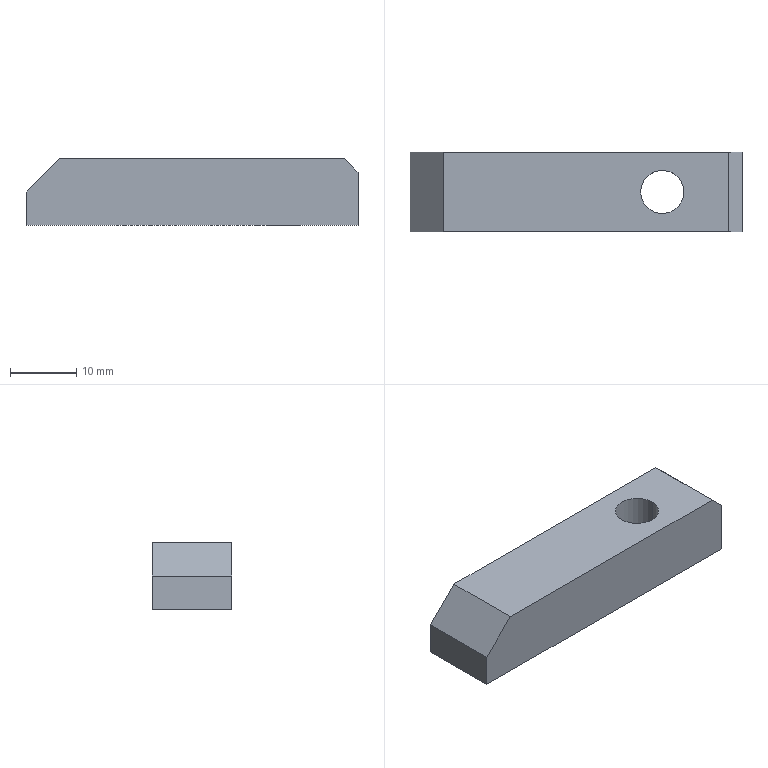Part | SolidWorks | features Chamfer 1, Extrusion 1, HoleWzd 1 | 1 solid | 10 faces | box 50 x 12 x 10 mm | volume 5494 mm3 | plane 8 | cylinder 2 | commonest cylinder face diameters 6.5 x2
STEP:
#1=CARTESIAN_POINT('',(9.75,0.,-5.));
#2=VERTEX_POINT('',#1);
#3=CARTESIAN_POINT('',(16.25,0.,-5.));
#4=VERTEX_POINT('',#3);
#5=CARTESIAN_POINT('',(13.,0.,-5.));
#6=DIRECTION('',(0.,0.,1.));
#7=DIRECTION('',(1.,0.,0.));
#8=AXIS2_PLACEMENT_3D('',#5,#6,#7);
#9=CIRCLE('',#8,3.25);
#10=EDGE_CURVE('',#2,#4,#9,.T.);
#11=ORIENTED_EDGE('',*,*,#10,.F.);
#12=CARTESIAN_POINT('',(9.75,0.,5.));
#13=VERTEX_POINT('',#12);
#14=CARTESIAN_POINT('',(9.75,0.,5.));
#15=DIRECTION('',(0.,0.,1.));
#16=VECTOR('',#15,1000.);
#17=LINE('',#14,#16);
#18=EDGE_CURVE('',#2,#13,#17,.T.);
#19=ORIENTED_EDGE('',*,*,#18,.T.);
#20=CARTESIAN_POINT('',(16.25,0.,5.));
#21=VERTEX_POINT('',#20);
#22=CARTESIAN_POINT('',(13.,0.,5.));
#23=DIRECTION('',(0.,0.,1.));
#24=DIRECTION('',(1.,0.,0.));
#25=AXIS2_PLACEMENT_3D('',#22,#23,#24);
#26=CIRCLE('',#25,3.25);
#27=EDGE_CURVE('',#13,#21,#26,.T.);
#28=ORIENTED_EDGE('',*,*,#27,.T.);
#29=CARTESIAN_POINT('',(16.25,0.,5.));
#30=DIRECTION('',(0.,0.,1.));
#31=VECTOR('',#30,1000.);
#32=LINE('',#29,#31);
#33=EDGE_CURVE('',#4,#21,#32,.T.);
#34=ORIENTED_EDGE('',*,*,#33,.F.);
#35=EDGE_LOOP('',(#11,#19,#28,#34));
#36=FACE_OUTER_BOUND('',#35,.T.);
#37=CARTESIAN_POINT('',(13.,0.,5.));
#38=DIRECTION('',(0.,0.,1.));
#39=DIRECTION('',(1.,0.,0.));
#40=AXIS2_PLACEMENT_3D('',#37,#38,#39);
#41=CYLINDRICAL_SURFACE('',#40,3.25);
#42=ADVANCED_FACE('',(#36),#41,.F.);
#43=CARTESIAN_POINT('',(-25.,6.,0.));
#44=VERTEX_POINT('',#43);
#45=CARTESIAN_POINT('',(-20.,6.,5.));
#46=VERTEX_POINT('',#45);
#47=CARTESIAN_POINT('',(-25.,6.,0.));
#48=DIRECTION('',(0.7071,0.,0.7071));
#49=VECTOR('',#48,1000.);
#50=LINE('',#47,#49);
#51=EDGE_CURVE('',#44,#46,#50,.T.);
#52=ORIENTED_EDGE('',*,*,#51,.F.);
#53=CARTESIAN_POINT('',(-25.,-6.,0.));
#54=VERTEX_POINT('',#53);
#55=CARTESIAN_POINT('',(-25.,-6.,0.));
#56=DIRECTION('',(0.,1.,0.));
#57=VECTOR('',#56,1000.);
#58=LINE('',#55,#57);
#59=EDGE_CURVE('',#54,#44,#58,.T.);
#60=ORIENTED_EDGE('',*,*,#59,.F.);
#61=CARTESIAN_POINT('',(-20.,-6.,5.));
#62=VERTEX_POINT('',#61);
#63=CARTESIAN_POINT('',(-25.,-6.,0.));
#64=DIRECTION('',(0.7071,0.,0.7071));
#65=VECTOR('',#64,1000.);
#66=LINE('',#63,#65);
#67=EDGE_CURVE('',#54,#62,#66,.T.);
#68=ORIENTED_EDGE('',*,*,#67,.T.);
#69=CARTESIAN_POINT('',(-20.,-6.,5.));
#70=DIRECTION('',(0.,1.,0.));
#71=VECTOR('',#70,1000.);
#72=LINE('',#69,#71);
#73=EDGE_CURVE('',#62,#46,#72,.T.);
#74=ORIENTED_EDGE('',*,*,#73,.T.);
#75=EDGE_LOOP('',(#52,#60,#68,#74));
#76=FACE_OUTER_BOUND('',#75,.T.);
#77=CARTESIAN_POINT('',(-25.,-6.,0.));
#78=DIRECTION('',(-0.7071,0.,0.7071));
#79=DIRECTION('',(0.7071,0.,0.7071));
#80=AXIS2_PLACEMENT_3D('',#77,#78,#79);
#81=PLANE('',#80);
#82=ADVANCED_FACE('',(#76),#81,.T.);
#83=CARTESIAN_POINT('',(-25.,6.,-5.));
#84=VERTEX_POINT('',#83);
#85=CARTESIAN_POINT('',(-25.,6.,-5.));
#86=DIRECTION('',(0.,0.,1.));
#87=VECTOR('',#86,1000.);
#88=LINE('',#85,#87);
#89=EDGE_CURVE('',#84,#44,#88,.T.);
#90=ORIENTED_EDGE('',*,*,#89,.F.);
#91=CARTESIAN_POINT('',(-25.,-6.,-5.));
#92=VERTEX_POINT('',#91);
#93=CARTESIAN_POINT('',(-25.,-6.,-5.));
#94=DIRECTION('',(0.,1.,0.));
#95=VECTOR('',#94,1000.);
#96=LINE('',#93,#95);
#97=EDGE_CURVE('',#92,#84,#96,.T.);
#98=ORIENTED_EDGE('',*,*,#97,.F.);
#99=CARTESIAN_POINT('',(-25.,-6.,-5.));
#100=DIRECTION('',(0.,0.,1.));
#101=VECTOR('',#100,1000.);
#102=LINE('',#99,#101);
#103=EDGE_CURVE('',#92,#54,#102,.T.);
#104=ORIENTED_EDGE('',*,*,#103,.T.);
#105=ORIENTED_EDGE('',*,*,#59,.T.);
#106=EDGE_LOOP('',(#90,#98,#104,#105));
#107=FACE_OUTER_BOUND('',#106,.T.);
#108=CARTESIAN_POINT('',(-25.,-6.,-5.));
#109=DIRECTION('',(-1.,0.,0.));
#110=DIRECTION('',(0.,0.,1.));
#111=AXIS2_PLACEMENT_3D('',#108,#109,#110);
#112=PLANE('',#111);
#113=ADVANCED_FACE('',(#107),#112,.T.);
#114=CARTESIAN_POINT('',(13.,0.,-5.));
#115=DIRECTION('',(0.,0.,1.));
#116=DIRECTION('',(1.,0.,0.));
#117=AXIS2_PLACEMENT_3D('',#114,#115,#116);
#118=CIRCLE('',#117,3.25);
#119=EDGE_CURVE('',#4,#2,#118,.T.);
#120=ORIENTED_EDGE('',*,*,#119,.T.);
#121=ORIENTED_EDGE('',*,*,#10,.T.);
#122=EDGE_LOOP('',(#120,#121));
#123=FACE_BOUND('',#122,.T.);
#124=CARTESIAN_POINT('',(25.,6.,-5.));
#125=VERTEX_POINT('',#124);
#126=CARTESIAN_POINT('',(25.,6.,-5.));
#127=DIRECTION('',(-1.,0.,0.));
#128=VECTOR('',#127,1000.);
#129=LINE('',#126,#128);
#130=EDGE_CURVE('',#125,#84,#129,.T.);
#131=ORIENTED_EDGE('',*,*,#130,.F.);
#132=CARTESIAN_POINT('',(25.,-6.,-5.));
#133=VERTEX_POINT('',#132);
#134=CARTESIAN_POINT('',(25.,-6.,-5.));
#135=DIRECTION('',(0.,1.,0.));
#136=VECTOR('',#135,1000.);
#137=LINE('',#134,#136);
#138=EDGE_CURVE('',#133,#125,#137,.T.);
#139=ORIENTED_EDGE('',*,*,#138,.F.);
#140=CARTESIAN_POINT('',(25.,-6.,-5.));
#141=DIRECTION('',(-1.,0.,0.));
#142=VECTOR('',#141,1000.);
#143=LINE('',#140,#142);
#144=EDGE_CURVE('',#133,#92,#143,.T.);
#145=ORIENTED_EDGE('',*,*,#144,.T.);
#146=ORIENTED_EDGE('',*,*,#97,.T.);
#147=EDGE_LOOP('',(#131,#139,#145,#146));
#148=FACE_OUTER_BOUND('',#147,.T.);
#149=CARTESIAN_POINT('',(25.,-6.,-5.));
#150=DIRECTION('',(0.,0.,-1.));
#151=DIRECTION('',(-1.,0.,0.));
#152=AXIS2_PLACEMENT_3D('',#149,#150,#151);
#153=PLANE('',#152);
#154=ADVANCED_FACE('',(#123,#148),#153,.T.);
#155=CARTESIAN_POINT('',(25.,6.,3.));
#156=VERTEX_POINT('',#155);
#157=CARTESIAN_POINT('',(25.,6.,5.));
#158=DIRECTION('',(0.,0.,-1.));
#159=VECTOR('',#158,1000.);
#160=LINE('',#157,#159);
#161=EDGE_CURVE('',#156,#125,#160,.T.);
#162=ORIENTED_EDGE('',*,*,#161,.F.);
#163=CARTESIAN_POINT('',(25.,-6.,3.));
#164=VERTEX_POINT('',#163);
#165=CARTESIAN_POINT('',(25.,-6.,3.));
#166=DIRECTION('',(0.,-1.,0.));
#167=VECTOR('',#166,1000.);
#168=LINE('',#165,#167);
#169=EDGE_CURVE('',#156,#164,#168,.T.);
#170=ORIENTED_EDGE('',*,*,#169,.T.);
#171=CARTESIAN_POINT('',(25.,-6.,5.));
#172=DIRECTION('',(0.,0.,-1.));
#173=VECTOR('',#172,1000.);
#174=LINE('',#171,#173);
#175=EDGE_CURVE('',#164,#133,#174,.T.);
#176=ORIENTED_EDGE('',*,*,#175,.T.);
#177=ORIENTED_EDGE('',*,*,#138,.T.);
#178=EDGE_LOOP('',(#162,#170,#176,#177));
#179=FACE_OUTER_BOUND('',#178,.T.);
#180=CARTESIAN_POINT('',(25.,-6.,5.));
#181=DIRECTION('',(1.,0.,0.));
#182=DIRECTION('',(0.,0.,-1.));
#183=AXIS2_PLACEMENT_3D('',#180,#181,#182);
#184=PLANE('',#183);
#185=ADVANCED_FACE('',(#179),#184,.T.);
#186=CARTESIAN_POINT('',(13.,0.,5.));
#187=DIRECTION('',(0.,0.,1.));
#188=DIRECTION('',(1.,0.,0.));
#189=AXIS2_PLACEMENT_3D('',#186,#187,#188);
#190=CIRCLE('',#189,3.25);
#191=EDGE_CURVE('',#21,#13,#190,.T.);
#192=ORIENTED_EDGE('',*,*,#191,.F.);
#193=ORIENTED_EDGE('',*,*,#27,.F.);
#194=EDGE_LOOP('',(#192,#193));
#195=FACE_BOUND('',#194,.T.);
#196=CARTESIAN_POINT('',(23.,-6.,5.));
#197=VERTEX_POINT('',#196);
#198=CARTESIAN_POINT('',(-20.,-6.,5.));
#199=DIRECTION('',(1.,0.,0.));
#200=VECTOR('',#199,1000.);
#201=LINE('',#198,#200);
#202=EDGE_CURVE('',#62,#197,#201,.T.);
#203=ORIENTED_EDGE('',*,*,#202,.T.);
#204=CARTESIAN_POINT('',(23.,6.,5.));
#205=VERTEX_POINT('',#204);
#206=CARTESIAN_POINT('',(23.,-6.,5.));
#207=DIRECTION('',(0.,1.,0.));
#208=VECTOR('',#207,1000.);
#209=LINE('',#206,#208);
#210=EDGE_CURVE('',#197,#205,#209,.T.);
#211=ORIENTED_EDGE('',*,*,#210,.T.);
#212=CARTESIAN_POINT('',(-20.,6.,5.));
#213=DIRECTION('',(1.,0.,0.));
#214=VECTOR('',#213,1000.);
#215=LINE('',#212,#214);
#216=EDGE_CURVE('',#46,#205,#215,.T.);
#217=ORIENTED_EDGE('',*,*,#216,.F.);
#218=ORIENTED_EDGE('',*,*,#73,.F.);
#219=EDGE_LOOP('',(#203,#211,#217,#218));
#220=FACE_OUTER_BOUND('',#219,.T.);
#221=CARTESIAN_POINT('',(-20.,-6.,5.));
#222=DIRECTION('',(0.,0.,1.));
#223=DIRECTION('',(1.,0.,0.));
#224=AXIS2_PLACEMENT_3D('',#221,#222,#223);
#225=PLANE('',#224);
#226=ADVANCED_FACE('',(#195,#220),#225,.T.);
#227=ORIENTED_EDGE('',*,*,#175,.F.);
#228=CARTESIAN_POINT('',(23.,-6.,5.));
#229=DIRECTION('',(-0.7071,0.,0.7071));
#230=VECTOR('',#229,1000.);
#231=LINE('',#228,#230);
#232=EDGE_CURVE('',#164,#197,#231,.T.);
#233=ORIENTED_EDGE('',*,*,#232,.T.);
#234=ORIENTED_EDGE('',*,*,#202,.F.);
#235=ORIENTED_EDGE('',*,*,#67,.F.);
#236=ORIENTED_EDGE('',*,*,#103,.F.);
#237=ORIENTED_EDGE('',*,*,#144,.F.);
#238=EDGE_LOOP('',(#227,#233,#234,#235,#236,#237));
#239=FACE_OUTER_BOUND('',#238,.T.);
#240=CARTESIAN_POINT('',(0.,-6.,0.));
#241=DIRECTION('',(0.,1.,0.));
#242=DIRECTION('',(0.,0.,1.));
#243=AXIS2_PLACEMENT_3D('',#240,#241,#242);
#244=PLANE('',#243);
#245=ADVANCED_FACE('',(#239),#244,.F.);
#246=ORIENTED_EDGE('',*,*,#216,.T.);
#247=CARTESIAN_POINT('',(14.,6.,14.));
#248=DIRECTION('',(0.7071,0.,-0.7071));
#249=VECTOR('',#248,1000.);
#250=LINE('',#247,#249);
#251=EDGE_CURVE('',#205,#156,#250,.T.);
#252=ORIENTED_EDGE('',*,*,#251,.T.);
#253=ORIENTED_EDGE('',*,*,#161,.T.);
#254=ORIENTED_EDGE('',*,*,#130,.T.);
#255=ORIENTED_EDGE('',*,*,#89,.T.);
#256=ORIENTED_EDGE('',*,*,#51,.T.);
#257=EDGE_LOOP('',(#246,#252,#253,#254,#255,#256));
#258=FACE_OUTER_BOUND('',#257,.T.);
#259=CARTESIAN_POINT('',(0.,6.,0.));
#260=DIRECTION('',(0.,1.,0.));
#261=DIRECTION('',(0.,0.,1.));
#262=AXIS2_PLACEMENT_3D('',#259,#260,#261);
#263=PLANE('',#262);
#264=ADVANCED_FACE('',(#258),#263,.T.);
#265=ORIENTED_EDGE('',*,*,#18,.F.);
#266=ORIENTED_EDGE('',*,*,#119,.F.);
#267=ORIENTED_EDGE('',*,*,#33,.T.);
#268=ORIENTED_EDGE('',*,*,#191,.T.);
#269=EDGE_LOOP('',(#265,#266,#267,#268));
#270=FACE_OUTER_BOUND('',#269,.T.);
#271=CARTESIAN_POINT('',(13.,0.,5.));
#272=DIRECTION('',(0.,0.,1.));
#273=DIRECTION('',(1.,0.,0.));
#274=AXIS2_PLACEMENT_3D('',#271,#272,#273);
#275=CYLINDRICAL_SURFACE('',#274,3.25);
#276=ADVANCED_FACE('',(#270),#275,.F.);
#277=ORIENTED_EDGE('',*,*,#232,.F.);
#278=ORIENTED_EDGE('',*,*,#169,.F.);
#279=ORIENTED_EDGE('',*,*,#251,.F.);
#280=ORIENTED_EDGE('',*,*,#210,.F.);
#281=EDGE_LOOP('',(#277,#278,#279,#280));
#282=FACE_OUTER_BOUND('',#281,.T.);
#283=CARTESIAN_POINT('',(23.,-6.,5.));
#284=DIRECTION('',(-0.7071,0.,-0.7071));
#285=DIRECTION('',(0.,1.,0.));
#286=AXIS2_PLACEMENT_3D('',#283,#284,#285);
#287=PLANE('',#286);
#288=ADVANCED_FACE('',(#282),#287,.F.);
#289=CLOSED_SHELL('',(#42,#82,#113,#154,#185,#226,#245,#264,#276,#288));
#290=MANIFOLD_SOLID_BREP('',#289);
#291=CARTESIAN_POINT('',(0.,0.,0.));
#292=DIRECTION('',(0.,0.,1.));
#293=DIRECTION('',(1.,0.,0.));
#294=AXIS2_PLACEMENT_3D('',#291,#292,#293);
#295=(LENGTH_UNIT()NAMED_UNIT(*)SI_UNIT(.MILLI.,.METRE.));
#296=UNCERTAINTY_MEASURE_WITH_UNIT(LENGTH_MEASURE(0.00001),#295,'','');
#297=(NAMED_UNIT(*)PLANE_ANGLE_UNIT()SI_UNIT($,.RADIAN.));
#298=(NAMED_UNIT(*)SI_UNIT($,.STERADIAN.)SOLID_ANGLE_UNIT());
#299=(GEOMETRIC_REPRESENTATION_CONTEXT(3)GLOBAL_UNCERTAINTY_ASSIGNED_CONTEXT((#296))GLOBAL_UNIT_ASSIGNED_CONTEXT((#295,#297,#298))REPRESENTATION_CONTEXT('',''));
#300=ADVANCED_BREP_SHAPE_REPRESENTATION('',(#290,#294),#299);